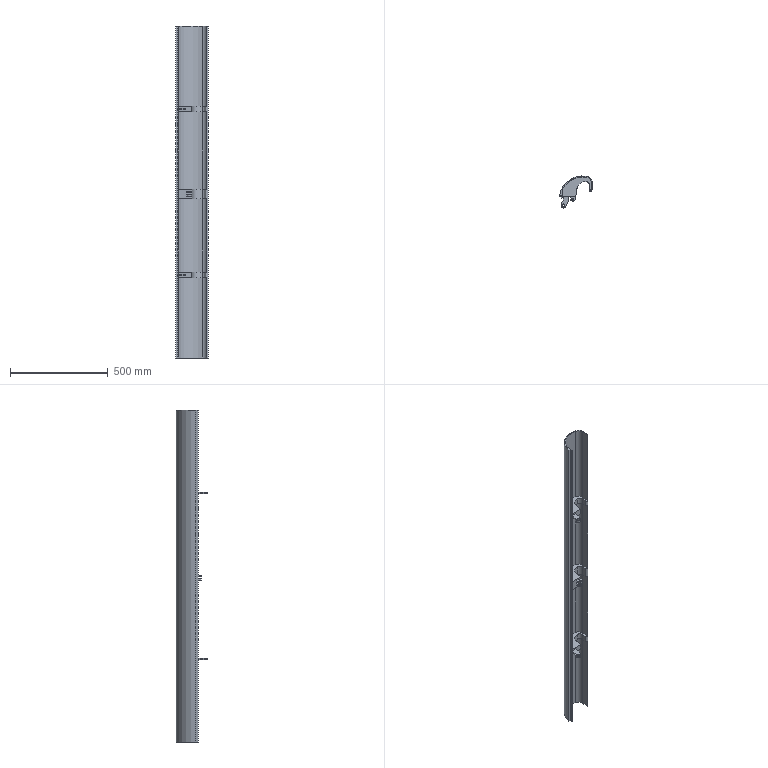Part | SolidWorks | features ICE 7, Extrusion 1 | 1 solid | 81 faces | box 168.561 x 162.568 x 1700 mm | volume 3528785 mm3 | cylinder 41 | plane 40 | commonest cylinder face diameters 58 x8 37 x5 10 x4 15 x4 228 x4 250 x4